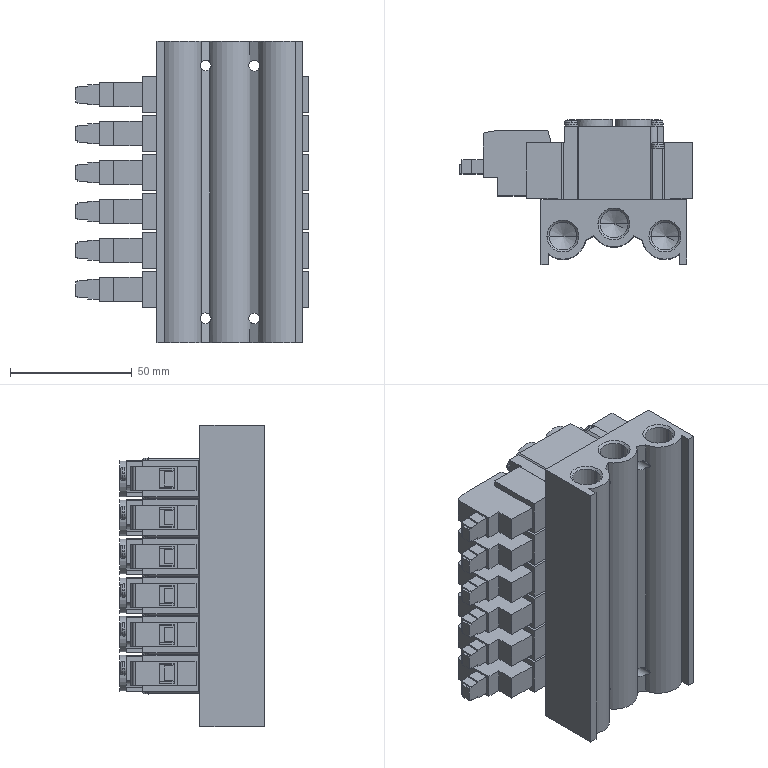Part | STEP file | SS5Y5-20-06_20-5LN-01_111111^Coding mechanism | 7 solids | 752 faces | box 95.8 x 59.5 x 124 mm | volume 347981 mm3 | plane 405 | cylinder 155 | cone 120 | torus 48 | sphere 24 | commonest cylinder face diameters 5.5 x48 8.566 x24 14.8 x24 5.8 x18 4.15 x12 11.445 x12